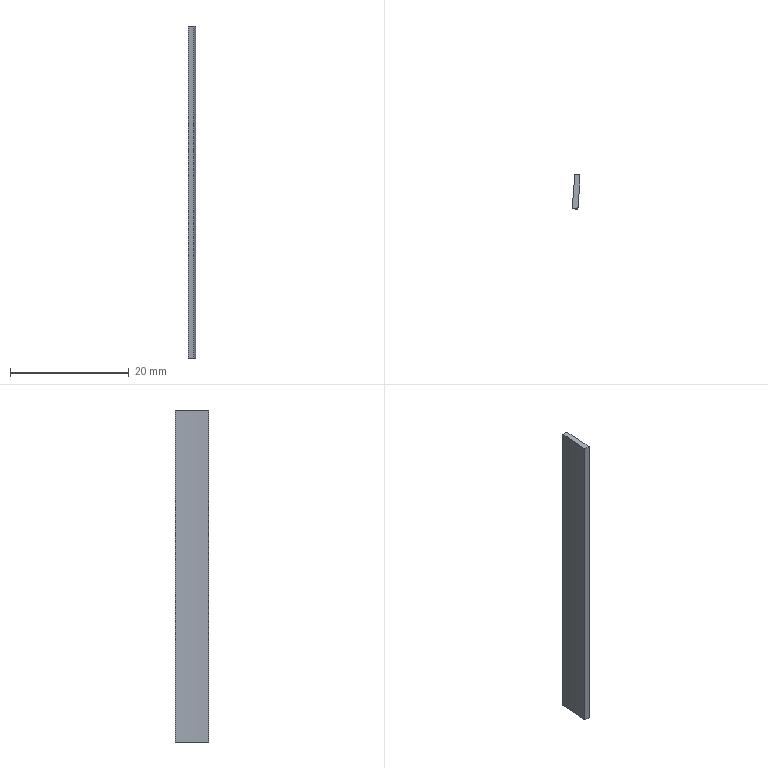Part | NX | features BREP 2 | 2 solids | 12 faces | box 1.335 x 5.733 x 56 mm | volume 600.481 mm3 | plane 8 | cylinder 4 | commonest cylinder face diameters 163.294 x2 188.049 x2
STEP:
#1=CARTESIAN_POINT('',(0.3386,-2.891,-4.));
#2=VERTEX_POINT('',#1);
#3=CARTESIAN_POINT('',(0.3386,-2.891,52.));
#4=VERTEX_POINT('',#3);
#5=CARTESIAN_POINT('',(0.3386,-2.891,0.));
#6=DIRECTION('',(0.,0.,1.));
#7=VECTOR('',#6,1000.);
#8=LINE('',#5,#7);
#9=EDGE_CURVE('',#2,#4,#8,.T.);
#10=ORIENTED_EDGE('',*,*,#9,.T.);
#11=CARTESIAN_POINT('',(-0.6423,-2.782,52.));
#12=VERTEX_POINT('',#11);
#13=CARTESIAN_POINT('',(-13.349,-1.37,52.));
#14=DIRECTION('',(0.9939,-0.1105,0.));
#15=VECTOR('',#14,1000.);
#16=LINE('',#13,#15);
#17=EDGE_CURVE('',#12,#4,#16,.T.);
#18=ORIENTED_EDGE('',*,*,#17,.F.);
#19=CARTESIAN_POINT('',(-0.6423,-2.782,-4.));
#20=VERTEX_POINT('',#19);
#21=CARTESIAN_POINT('',(-0.6423,-2.782,0.));
#22=DIRECTION('',(0.,0.,1.));
#23=VECTOR('',#22,1000.);
#24=LINE('',#21,#23);
#25=EDGE_CURVE('',#20,#12,#24,.T.);
#26=ORIENTED_EDGE('',*,*,#25,.F.);
#27=CARTESIAN_POINT('',(-13.349,-1.37,-4.));
#28=DIRECTION('',(0.9939,-0.1105,0.));
#29=VECTOR('',#28,1000.);
#30=LINE('',#27,#29);
#31=EDGE_CURVE('',#20,#2,#30,.T.);
#32=ORIENTED_EDGE('',*,*,#31,.T.);
#33=EDGE_LOOP('',(#10,#18,#26,#32));
#34=FACE_BOUND('',#33,.T.);
#35=CARTESIAN_POINT('',(-13.349,-1.37,0.));
#36=DIRECTION('',(-0.1105,-0.9939,0.));
#37=DIRECTION('',(-0.9939,0.1105,0.));
#38=AXIS2_PLACEMENT_3D('',#35,#36,#37);
#39=PLANE('',#38);
#40=ADVANCED_FACE('',(#34),#39,.T.);
#41=ORIENTED_EDGE('',*,*,#25,.T.);
#42=CARTESIAN_POINT('',(-0.213,2.841,52.));
#43=VERTEX_POINT('',#42);
#44=CARTESIAN_POINT('',(-81.789,6.24,52.));
#45=DIRECTION('',(0.,0.,-1.));
#46=DIRECTION('',(1.,0.,0.));
#47=AXIS2_PLACEMENT_3D('',#44,#45,#46);
#48=CIRCLE('',#47,81.647);
#49=EDGE_CURVE('',#43,#12,#48,.T.);
#50=ORIENTED_EDGE('',*,*,#49,.F.);
#51=CARTESIAN_POINT('',(-0.213,2.841,-4.));
#52=VERTEX_POINT('',#51);
#53=CARTESIAN_POINT('',(-0.213,2.841,0.));
#54=DIRECTION('',(0.,0.,1.));
#55=VECTOR('',#54,1000.);
#56=LINE('',#53,#55);
#57=EDGE_CURVE('',#52,#43,#56,.T.);
#58=ORIENTED_EDGE('',*,*,#57,.F.);
#59=CARTESIAN_POINT('',(-81.789,6.24,-4.));
#60=DIRECTION('',(0.,0.,-1.));
#61=DIRECTION('',(1.,0.,0.));
#62=AXIS2_PLACEMENT_3D('',#59,#60,#61);
#63=CIRCLE('',#62,81.647);
#64=EDGE_CURVE('',#52,#20,#63,.T.);
#65=ORIENTED_EDGE('',*,*,#64,.T.);
#66=EDGE_LOOP('',(#41,#50,#58,#65));
#67=FACE_BOUND('',#66,.T.);
#68=CARTESIAN_POINT('',(-81.789,6.24,0.));
#69=DIRECTION('',(0.,0.,1.));
#70=DIRECTION('',(-1.,0.,0.));
#71=AXIS2_PLACEMENT_3D('',#68,#69,#70);
#72=CYLINDRICAL_SURFACE('',#71,81.647);
#73=ADVANCED_FACE('',(#67),#72,.F.);
#74=ORIENTED_EDGE('',*,*,#57,.T.);
#75=CARTESIAN_POINT('',(0.6923,2.841,52.));
#76=VERTEX_POINT('',#75);
#77=CARTESIAN_POINT('',(-12.323,2.841,52.));
#78=DIRECTION('',(-1.,0.,0.));
#79=VECTOR('',#78,1000.);
#80=LINE('',#77,#79);
#81=EDGE_CURVE('',#76,#43,#80,.T.);
#82=ORIENTED_EDGE('',*,*,#81,.F.);
#83=CARTESIAN_POINT('',(0.6923,2.841,-4.));
#84=VERTEX_POINT('',#83);
#85=CARTESIAN_POINT('',(0.6923,2.841,0.));
#86=DIRECTION('',(0.,0.,1.));
#87=VECTOR('',#86,1000.);
#88=LINE('',#85,#87);
#89=EDGE_CURVE('',#84,#76,#88,.T.);
#90=ORIENTED_EDGE('',*,*,#89,.F.);
#91=CARTESIAN_POINT('',(-12.323,2.841,-4.));
#92=DIRECTION('',(-1.,0.,0.));
#93=VECTOR('',#92,1000.);
#94=LINE('',#91,#93);
#95=EDGE_CURVE('',#84,#52,#94,.T.);
#96=ORIENTED_EDGE('',*,*,#95,.T.);
#97=EDGE_LOOP('',(#74,#82,#90,#96));
#98=FACE_BOUND('',#97,.T.);
#99=CARTESIAN_POINT('',(-12.323,2.841,0.));
#100=DIRECTION('',(0.,-1.,0.));
#101=DIRECTION('',(-1.,0.,0.));
#102=AXIS2_PLACEMENT_3D('',#99,#100,#101);
#103=PLANE('',#102);
#104=ADVANCED_FACE('',(#98),#103,.F.);
#105=CARTESIAN_POINT('',(-93.287,5.761,-4.));
#106=DIRECTION('',(0.,0.,1.));
#107=DIRECTION('',(1.,0.,0.));
#108=AXIS2_PLACEMENT_3D('',#105,#106,#107);
#109=CIRCLE('',#108,94.024);
#110=EDGE_CURVE('',#2,#84,#109,.T.);
#111=ORIENTED_EDGE('',*,*,#110,.T.);
#112=ORIENTED_EDGE('',*,*,#89,.T.);
#113=CARTESIAN_POINT('',(-93.287,5.761,52.));
#114=DIRECTION('',(0.,0.,1.));
#115=DIRECTION('',(1.,0.,0.));
#116=AXIS2_PLACEMENT_3D('',#113,#114,#115);
#117=CIRCLE('',#116,94.024);
#118=EDGE_CURVE('',#4,#76,#117,.T.);
#119=ORIENTED_EDGE('',*,*,#118,.F.);
#120=ORIENTED_EDGE('',*,*,#9,.F.);
#121=EDGE_LOOP('',(#111,#112,#119,#120));
#122=FACE_BOUND('',#121,.T.);
#123=CARTESIAN_POINT('',(-93.287,5.761,0.));
#124=DIRECTION('',(0.,0.,1.));
#125=DIRECTION('',(-1.,0.,0.));
#126=AXIS2_PLACEMENT_3D('',#123,#124,#125);
#127=CYLINDRICAL_SURFACE('',#126,94.024);
#128=ADVANCED_FACE('',(#122),#127,.T.);
#129=ORIENTED_EDGE('',*,*,#81,.T.);
#130=ORIENTED_EDGE('',*,*,#49,.T.);
#131=ORIENTED_EDGE('',*,*,#17,.T.);
#132=ORIENTED_EDGE('',*,*,#118,.T.);
#133=EDGE_LOOP('',(#129,#130,#131,#132));
#134=FACE_BOUND('',#133,.T.);
#135=CARTESIAN_POINT('',(-12.323,7.857,52.));
#136=DIRECTION('',(0.,0.,1.));
#137=DIRECTION('',(-1.,0.,0.));
#138=AXIS2_PLACEMENT_3D('',#135,#136,#137);
#139=PLANE('',#138);
#140=ADVANCED_FACE('',(#134),#139,.T.);
#141=ORIENTED_EDGE('',*,*,#95,.F.);
#142=ORIENTED_EDGE('',*,*,#110,.F.);
#143=ORIENTED_EDGE('',*,*,#31,.F.);
#144=ORIENTED_EDGE('',*,*,#64,.F.);
#145=EDGE_LOOP('',(#141,#142,#143,#144));
#146=FACE_BOUND('',#145,.T.);
#147=CARTESIAN_POINT('',(-12.323,7.857,-4.));
#148=DIRECTION('',(0.,0.,1.));
#149=DIRECTION('',(-1.,0.,0.));
#150=AXIS2_PLACEMENT_3D('',#147,#148,#149);
#151=PLANE('',#150);
#152=ADVANCED_FACE('',(#146),#151,.F.);
#153=CLOSED_SHELL('',(#40,#73,#104,#128,#140,#152));
#154=MANIFOLD_SOLID_BREP('',#153);
#155=CARTESIAN_POINT('',(0.3386,-2.891,-4.));
#156=VERTEX_POINT('',#155);
#157=CARTESIAN_POINT('',(0.3386,-2.891,52.));
#158=VERTEX_POINT('',#157);
#159=CARTESIAN_POINT('',(0.3386,-2.891,0.));
#160=DIRECTION('',(0.,0.,1.));
#161=VECTOR('',#160,1000.);
#162=LINE('',#159,#161);
#163=EDGE_CURVE('',#156,#158,#162,.T.);
#164=ORIENTED_EDGE('',*,*,#163,.T.);
#165=CARTESIAN_POINT('',(-0.6423,-2.782,52.));
#166=VERTEX_POINT('',#165);
#167=CARTESIAN_POINT('',(-13.349,-1.37,52.));
#168=DIRECTION('',(0.9939,-0.1105,0.));
#169=VECTOR('',#168,1000.);
#170=LINE('',#167,#169);
#171=EDGE_CURVE('',#166,#158,#170,.T.);
#172=ORIENTED_EDGE('',*,*,#171,.F.);
#173=CARTESIAN_POINT('',(-0.6423,-2.782,-4.));
#174=VERTEX_POINT('',#173);
#175=CARTESIAN_POINT('',(-0.6423,-2.782,0.));
#176=DIRECTION('',(0.,0.,1.));
#177=VECTOR('',#176,1000.);
#178=LINE('',#175,#177);
#179=EDGE_CURVE('',#174,#166,#178,.T.);
#180=ORIENTED_EDGE('',*,*,#179,.F.);
#181=CARTESIAN_POINT('',(-13.349,-1.37,-4.));
#182=DIRECTION('',(0.9939,-0.1105,0.));
#183=VECTOR('',#182,1000.);
#184=LINE('',#181,#183);
#185=EDGE_CURVE('',#174,#156,#184,.T.);
#186=ORIENTED_EDGE('',*,*,#185,.T.);
#187=EDGE_LOOP('',(#164,#172,#180,#186));
#188=FACE_BOUND('',#187,.T.);
#189=CARTESIAN_POINT('',(-13.349,-1.37,0.));
#190=DIRECTION('',(-0.1105,-0.9939,0.));
#191=DIRECTION('',(-0.9939,0.1105,0.));
#192=AXIS2_PLACEMENT_3D('',#189,#190,#191);
#193=PLANE('',#192);
#194=ADVANCED_FACE('',(#188),#193,.T.);
#195=ORIENTED_EDGE('',*,*,#179,.T.);
#196=CARTESIAN_POINT('',(-0.213,2.841,52.));
#197=VERTEX_POINT('',#196);
#198=CARTESIAN_POINT('',(-81.789,6.24,52.));
#199=DIRECTION('',(0.,0.,-1.));
#200=DIRECTION('',(1.,0.,0.));
#201=AXIS2_PLACEMENT_3D('',#198,#199,#200);
#202=CIRCLE('',#201,81.647);
#203=EDGE_CURVE('',#197,#166,#202,.T.);
#204=ORIENTED_EDGE('',*,*,#203,.F.);
#205=CARTESIAN_POINT('',(-0.213,2.841,-4.));
#206=VERTEX_POINT('',#205);
#207=CARTESIAN_POINT('',(-0.213,2.841,0.));
#208=DIRECTION('',(0.,0.,1.));
#209=VECTOR('',#208,1000.);
#210=LINE('',#207,#209);
#211=EDGE_CURVE('',#206,#197,#210,.T.);
#212=ORIENTED_EDGE('',*,*,#211,.F.);
#213=CARTESIAN_POINT('',(-81.789,6.24,-4.));
#214=DIRECTION('',(0.,0.,-1.));
#215=DIRECTION('',(1.,0.,0.));
#216=AXIS2_PLACEMENT_3D('',#213,#214,#215);
#217=CIRCLE('',#216,81.647);
#218=EDGE_CURVE('',#206,#174,#217,.T.);
#219=ORIENTED_EDGE('',*,*,#218,.T.);
#220=EDGE_LOOP('',(#195,#204,#212,#219));
#221=FACE_BOUND('',#220,.T.);
#222=CARTESIAN_POINT('',(-81.789,6.24,0.));
#223=DIRECTION('',(0.,0.,1.));
#224=DIRECTION('',(-1.,0.,0.));
#225=AXIS2_PLACEMENT_3D('',#222,#223,#224);
#226=CYLINDRICAL_SURFACE('',#225,81.647);
#227=ADVANCED_FACE('',(#221),#226,.F.);
#228=ORIENTED_EDGE('',*,*,#211,.T.);
#229=CARTESIAN_POINT('',(0.6923,2.841,52.));
#230=VERTEX_POINT('',#229);
#231=CARTESIAN_POINT('',(-12.323,2.841,52.));
#232=DIRECTION('',(-1.,0.,0.));
#233=VECTOR('',#232,1000.);
#234=LINE('',#231,#233);
#235=EDGE_CURVE('',#230,#197,#234,.T.);
#236=ORIENTED_EDGE('',*,*,#235,.F.);
#237=CARTESIAN_POINT('',(0.6923,2.841,-4.));
#238=VERTEX_POINT('',#237);
#239=CARTESIAN_POINT('',(0.6923,2.841,0.));
#240=DIRECTION('',(0.,0.,1.));
#241=VECTOR('',#240,1000.);
#242=LINE('',#239,#241);
#243=EDGE_CURVE('',#238,#230,#242,.T.);
#244=ORIENTED_EDGE('',*,*,#243,.F.);
#245=CARTESIAN_POINT('',(-12.323,2.841,-4.));
#246=DIRECTION('',(-1.,0.,0.));
#247=VECTOR('',#246,1000.);
#248=LINE('',#245,#247);
#249=EDGE_CURVE('',#238,#206,#248,.T.);
#250=ORIENTED_EDGE('',*,*,#249,.T.);
#251=EDGE_LOOP('',(#228,#236,#244,#250));
#252=FACE_BOUND('',#251,.T.);
#253=CARTESIAN_POINT('',(-12.323,2.841,0.));
#254=DIRECTION('',(0.,-1.,0.));
#255=DIRECTION('',(-1.,0.,0.));
#256=AXIS2_PLACEMENT_3D('',#253,#254,#255);
#257=PLANE('',#256);
#258=ADVANCED_FACE('',(#252),#257,.F.);
#259=CARTESIAN_POINT('',(-93.287,5.761,-4.));
#260=DIRECTION('',(0.,0.,1.));
#261=DIRECTION('',(1.,0.,0.));
#262=AXIS2_PLACEMENT_3D('',#259,#260,#261);
#263=CIRCLE('',#262,94.024);
#264=EDGE_CURVE('',#156,#238,#263,.T.);
#265=ORIENTED_EDGE('',*,*,#264,.T.);
#266=ORIENTED_EDGE('',*,*,#243,.T.);
#267=CARTESIAN_POINT('',(-93.287,5.761,52.));
#268=DIRECTION('',(0.,0.,1.));
#269=DIRECTION('',(1.,0.,0.));
#270=AXIS2_PLACEMENT_3D('',#267,#268,#269);
#271=CIRCLE('',#270,94.024);
#272=EDGE_CURVE('',#158,#230,#271,.T.);
#273=ORIENTED_EDGE('',*,*,#272,.F.);
#274=ORIENTED_EDGE('',*,*,#163,.F.);
#275=EDGE_LOOP('',(#265,#266,#273,#274));
#276=FACE_BOUND('',#275,.T.);
#277=CARTESIAN_POINT('',(-93.287,5.761,0.));
#278=DIRECTION('',(0.,0.,1.));
#279=DIRECTION('',(-1.,0.,0.));
#280=AXIS2_PLACEMENT_3D('',#277,#278,#279);
#281=CYLINDRICAL_SURFACE('',#280,94.024);
#282=ADVANCED_FACE('',(#276),#281,.T.);
#283=ORIENTED_EDGE('',*,*,#235,.T.);
#284=ORIENTED_EDGE('',*,*,#203,.T.);
#285=ORIENTED_EDGE('',*,*,#171,.T.);
#286=ORIENTED_EDGE('',*,*,#272,.T.);
#287=EDGE_LOOP('',(#283,#284,#285,#286));
#288=FACE_BOUND('',#287,.T.);
#289=CARTESIAN_POINT('',(-12.323,7.857,52.));
#290=DIRECTION('',(0.,0.,1.));
#291=DIRECTION('',(-1.,0.,0.));
#292=AXIS2_PLACEMENT_3D('',#289,#290,#291);
#293=PLANE('',#292);
#294=ADVANCED_FACE('',(#288),#293,.T.);
#295=ORIENTED_EDGE('',*,*,#249,.F.);
#296=ORIENTED_EDGE('',*,*,#264,.F.);
#297=ORIENTED_EDGE('',*,*,#185,.F.);
#298=ORIENTED_EDGE('',*,*,#218,.F.);
#299=EDGE_LOOP('',(#295,#296,#297,#298));
#300=FACE_BOUND('',#299,.T.);
#301=CARTESIAN_POINT('',(-12.323,7.857,-4.));
#302=DIRECTION('',(0.,0.,1.));
#303=DIRECTION('',(-1.,0.,0.));
#304=AXIS2_PLACEMENT_3D('',#301,#302,#303);
#305=PLANE('',#304);
#306=ADVANCED_FACE('',(#300),#305,.F.);
#307=CLOSED_SHELL('',(#194,#227,#258,#282,#294,#306));
#308=MANIFOLD_SOLID_BREP('',#307);
#309=(LENGTH_UNIT()NAMED_UNIT(*)SI_UNIT(.MILLI.,.METRE.));
#310=UNCERTAINTY_MEASURE_WITH_UNIT(LENGTH_MEASURE(0.00001),#309,'','');
#311=(NAMED_UNIT(*)PLANE_ANGLE_UNIT()SI_UNIT($,.RADIAN.));
#312=(NAMED_UNIT(*)SI_UNIT($,.STERADIAN.)SOLID_ANGLE_UNIT());
#313=(GEOMETRIC_REPRESENTATION_CONTEXT(3)GLOBAL_UNCERTAINTY_ASSIGNED_CONTEXT((#310))GLOBAL_UNIT_ASSIGNED_CONTEXT((#309,#311,#312))REPRESENTATION_CONTEXT('',''));
#314=ADVANCED_BREP_SHAPE_REPRESENTATION('',(#154,#308),#313);